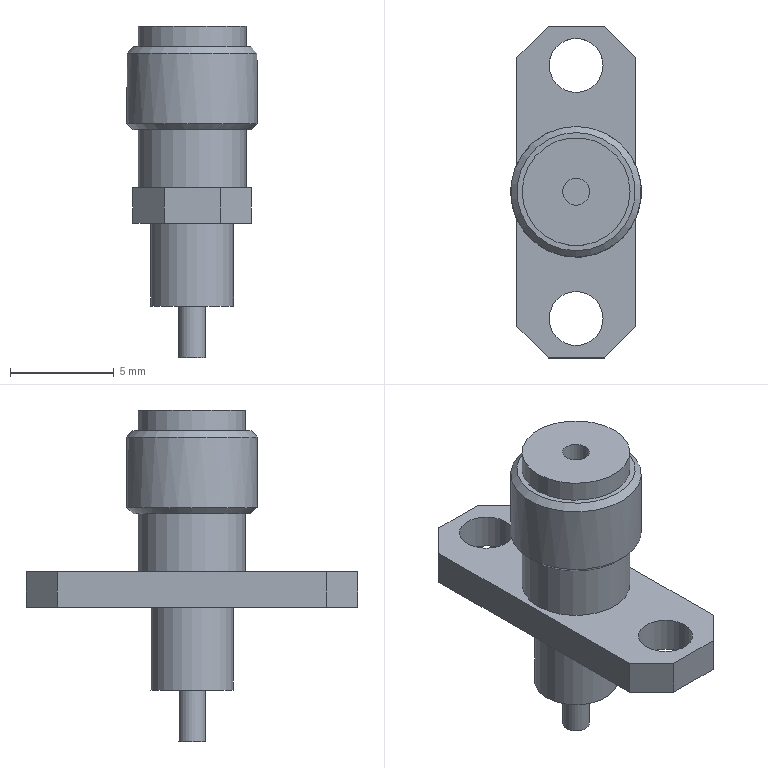Part | STEP file | Connector SMA-KFD561 | 1 solid | 26 faces | box 6.3 x 16 x 16 mm | volume 381.279 mm3 | plane 16 | cylinder 8 | cone 2 | commonest cylinder face diameters 1.3 x2 2.6 x2 5.2 x2 4 x1 6.3 x1